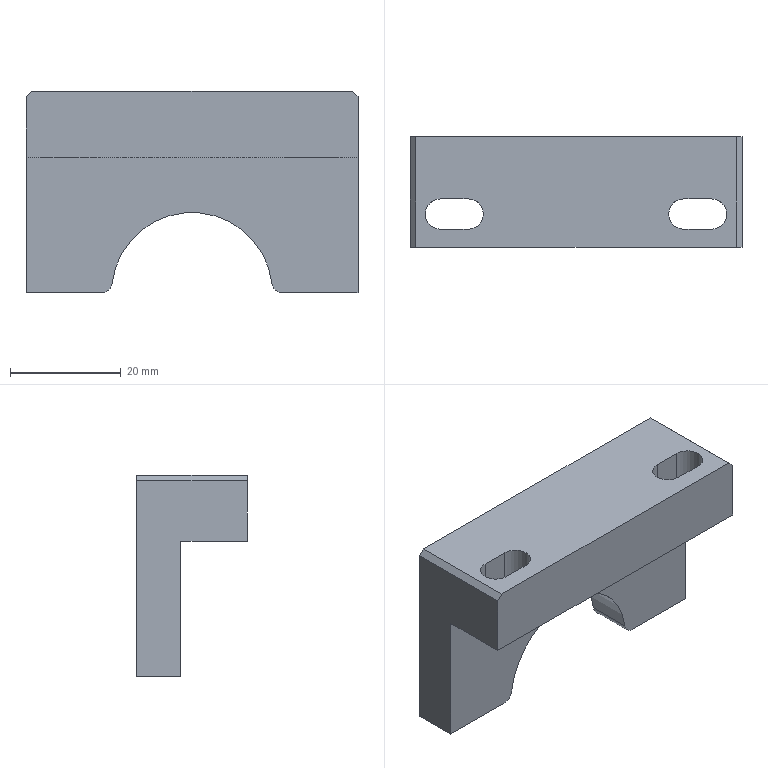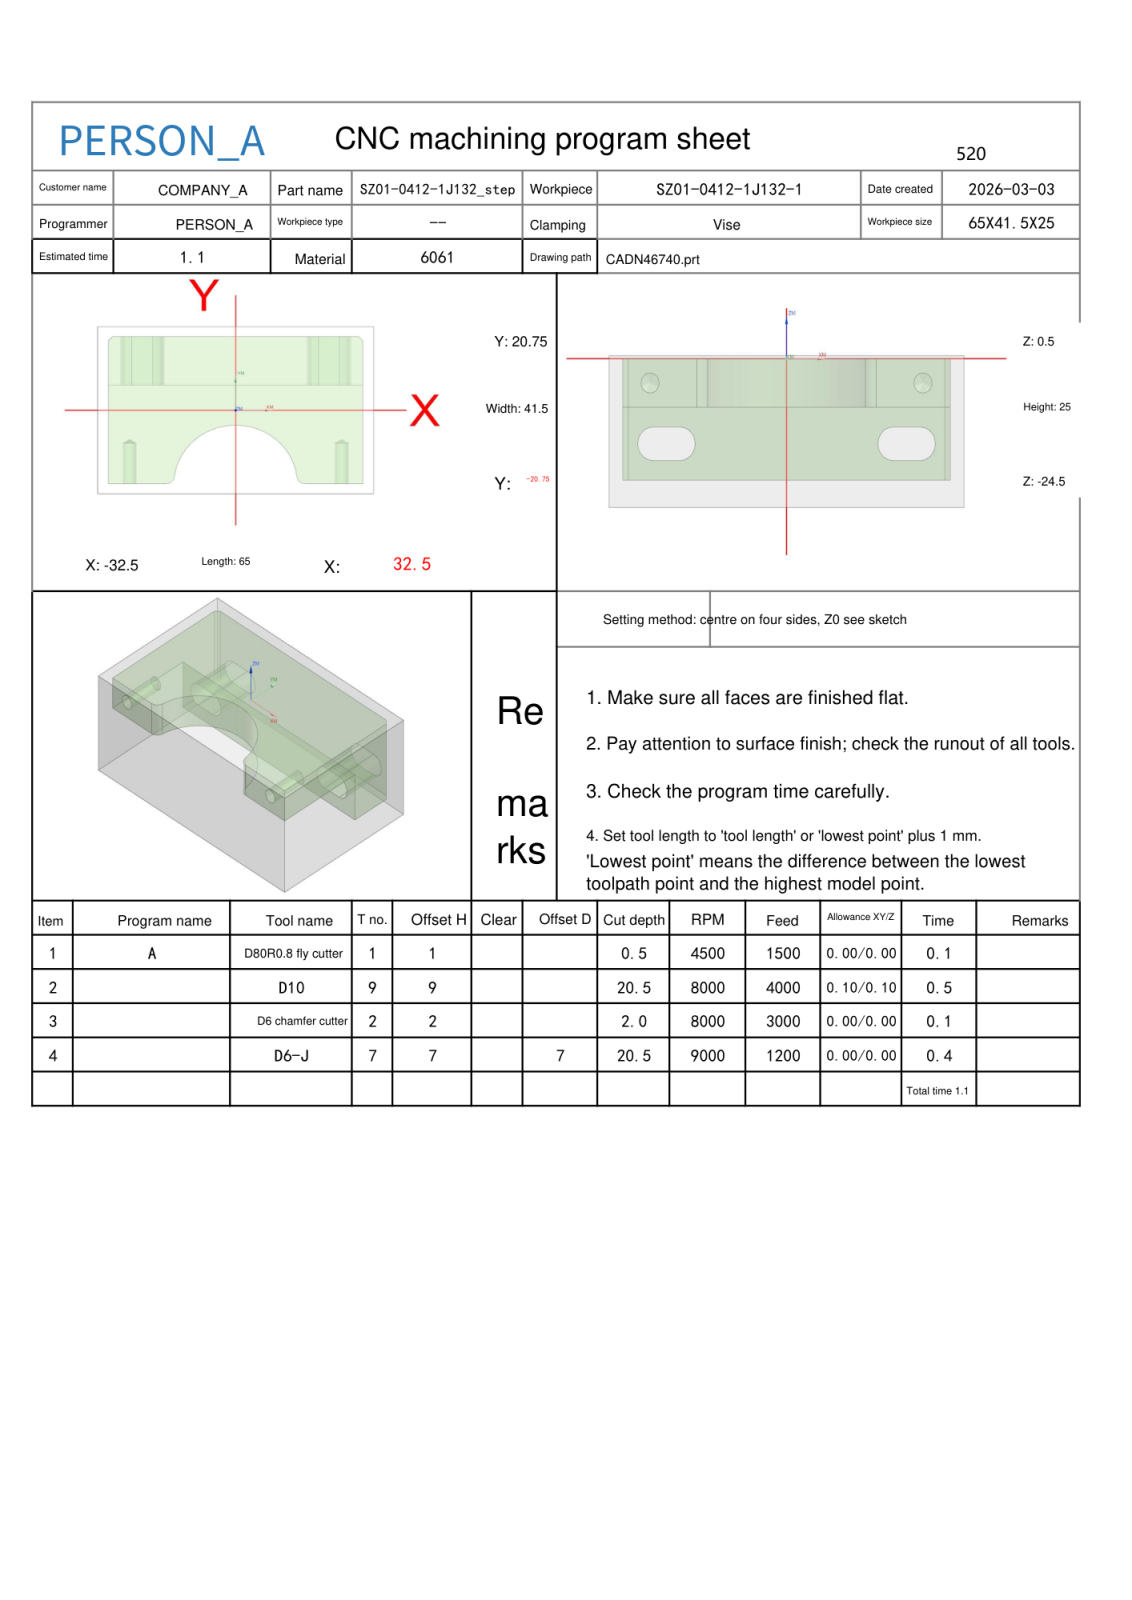NC program | NX | posted by the shop | part box 60 x 20 x 36.5 mm
Whole program:
%
O0001
(Machine time: 1.86 MIN)
(===Total Tool:4===)
(T1=D80R0.8 fly cutter D=80.  R=0.8  D-  H01 Z=0.    )
(T9=D10     D=10.  R=0.   D-  H09 Z=-20.  )
(T2=D6 chamfer cutter   D=6.   R=0.   D-  H02 Z=-1.5  )
(T7=D6-J    D=6.   R=0.   D7  H07 Z=-20.  )
G80 G90 G17 G49 G40
G91 G28 Z0
M01
N1 T01 M06
(D80R0.8 fly cutter  D=80. R=0.8 H=01 ce=0.00 di=0.00)
G00 G90 G54 X-75. Y0.0 M03 S4500
G43 H01 Z50.
M08
Z2.
G01 Z0.0 F1500.
X-70.
X70.
X75.
Z2.
G00 Z50.
G91 G28 Z0.0
M05
M09
G91 G28 Z0.0
M01
N2 T09 M06
(D10  D=10. R=0. H=09 ce=0.10 di=0.10)
G00 G90 G54 X-1.014 Y31.181 M03 S8000
G43 H09 Z50.
M08
Z-18.
G01 X-.995 Y31.082 Z-18.625 F4000.
X-.977 Y30.984 Z-18.872
X-.958 Y30.886 Z-19.054
X-.939 Y30.788 Z-19.2
X-.921 Y30.689 Z-19.323
X-.902 Y30.591 Z-19.428
X-.883 Y30.493 Z-19.52
X-.865 Y30.395 Z-19.6
X-.846 Y30.296 Z-19.67
X-.827 Y30.198 Z-19.732
X-.809 Y30.1 Z-19.786
X-.79 Y30.002 Z-19.833
X-.771 Y29.903 Z-19.874
X-.753 Y29.805 Z-19.908
X-.734 Y29.707 Z-19.936
X-.715 Y29.609 Z-19.96
X-.697 Y29.511 Z-19.977
X-.678 Y29.412 Z-19.99
X-.659 Y29.314 Z-19.997
X-.641 Y29.216 Z-20.
X-.239 Y27.102
G03 X.02 Y26.75 I.505 J.101
X3.834 Y26.112 I4.014 J12.271
X14.004 Y25.931 I10.17 J285.72
X17.328 Y25.95 I0.0 J285.901
G02 X22.505 Y25.974 I5.176 J-566.013
X30.847 Y25.912 I0.0 J-566.037
X35.808 Y22.571 I-.576 J-6.208
X37.387 Y16.992 I-12.592 J-6.578
X37.711 Y8.503 I-111.018 J-8.489
X37.695 Y6.6 I-111.342 J0.0
G01 X37.676 Y-18.9
G02 X34.409 Y-23.999 I-6.192 J.371
X28.685 Y-25.642 I-6.663 J12.425
X20.198 Y-25.962 I-8.487 J112.43
X18.294 Y-25.945 I0.0 J112.75
G01 X-30.63 Y-25.928
G02 X-35.719 Y-22.702 I.352 J6.181
X-37.387 Y-16.973 I12.246 J6.672
X-37.7 Y-9.187 I96.703 J7.786
X-37.692 Y-7.942 I97.015 J0.0
G01 X-37.676 Y18.9
G02 X-34.447 Y23.972 I6.185 J-.374
X-28.889 Y25.618 I6.599 J-12.074
X-20.788 Y25.956 I8.1 J-97.034
X-19.218 Y25.943 I0.0 J-97.371
X-12.284 Y25.971 I6.934 J-881.187
X-2.439 Y25.916 I0.0 J-881.214
G03 X6.567 Y25.245 I14.435 J133.079
X21.95 Y25.126 I15.383 J989.867
X28.108 Y25.145 I0.0 J989.986
G02 X34.603 Y21.21 I-.184 J-7.63
X36.473 Y15.222 I-13.036 J-7.357
X36.899 Y6.533 I-88.401 J-8.69
X36.888 Y5.156 I-88.827 J0.0
G01 X36.878 Y-16.757
G02 X32.777 Y-22.959 I-7.676 J.618
X26.519 Y-24.774 I-7.551 J14.34
X17.602 Y-25.155 I-8.918 J104.227
X15.971 Y-25.142 I0.0 J104.608
G01 X-28.487 Y-25.129
G02 X-34.704 Y-21.033 I.6 J7.678
X-36.532 Y-14.698 I14.384 J7.582
X-36.904 Y-5.801 I106.207 J8.896
X-36.893 Y-4.229 I106.579 J0.0
G01 X-36.879 Y16.737
G02 X-33.057 Y22.788 I7.611 J-.575
X-27.079 Y24.708 I7.365 J-12.666
X-19.035 Y25.132 I8.044 J-75.929
X-18.294 Y25.129 I0.0 J-76.354
X-11.995 Y25.164 I6.3 J-560.555
X-3.675 Y25.103 I0.0 J-560.59
G03 X6.265 Y24.482 I27.961 J367.714
X22.104 Y24.326 I15.839 J805.883
X26.268 Y24.337 I0.0 J806.039
G02 X30.598 Y23.063 I-.108 J-8.365
X32.829 Y21.648 I-1.556 J-4.922
X34.641 Y19.364 I-5.043 J-5.86
X35.582 Y14.955 I-17.95 J-6.134
X36.112 Y4.461 I-103.61 J-10.494
X36.093 Y2.493 I-104.14 J0.0
X36.121 Y-4.832 I-944.209 J-7.326
X36.068 Y-14.846 I-944.237 J0.0
X35.073 Y-18.453 I-8.82 J.492
G01 X34.926 Y-19.57
X34.417 Y-20.8
X33.606 Y-21.856
X32.55 Y-22.667
X31.32 Y-23.176
G02 X19.21 Y-24.313 I-12.83 J71.616
G01 X8.331 Y-24.349
X-26.289 Y-24.333
G02 X-30.191 Y-23.325 I.171 J8.716
G01 X-31.32 Y-23.176
X-32.55 Y-22.667
X-33.606 Y-21.856
X-34.417 Y-20.8
G02 X-35.145 Y-18.268 I6.23 J3.162
X-36.057 Y-7.678 I70.414 J11.403
G01 X-36.099 Y4.241
G02 X-36.123 Y8.231 I332.132 J3.99
X-36.052 Y15.1 I332.156 J0.0
X-34.818 Y18.836 I8.257 J-.655
X-33.606 Y20.857 I4.477 J-1.312
X-31.486 Y22.703 I7.177 J-6.102
X-28.417 Y23.572 I4.288 J-9.287
X-19.095 Y24.312 I9.951 J-66.268
X-12.541 Y24.363 I6.554 J-421.66
X-3.416 Y24.264 I0.0 J-421.711
G03 X15.543 Y23.546 I18.959 J249.717
X17.735 Y23.555 I0.0 J250.435
G02 X20.074 Y23.572 I2.339 J-160.329
X25.168 Y23.491 I0.0 J-160.346
G01 X26.223 Y23.35
X29.025
X30.297 Y23.185
X30.668 Y23.035
X30.297 Y23.185
X29.025 Y23.35
X1.555 Y23.373
G03 X-11.967 Y23.724 I-13.522 J-260.677
X-22.674 Y23.504 I0.0 J-261.028
G01 X-24.721 Y23.35
X-29.023
X-30.297 Y23.185
X-29.023 Y23.35
X2.399
G03 X2.779 Y23.525 I-.006 J.513
G01 X3.45 Y24.312
X4.729 Y25.812 Z-19.9
X5.155 Y26.311
X5.217 Y26.372
X5.288 Y26.421
X5.366 Y26.457
X5.45 Y26.479
X5.536 Y26.487
X31.253
X31.455 Y26.48
X31.656 Y26.461
X31.855 Y26.429
X32.051 Y26.384
X32.245 Y26.326
X32.434 Y26.256
X32.618 Y26.174
X32.797 Y26.081
X32.969 Y25.976
X33.134 Y25.86
X33.292 Y25.734
X33.441 Y25.598
X33.581 Y25.452
X36.132 Y22.626
X36.178 Y22.566
X36.215 Y22.5
X36.242 Y22.428
X36.257 Y22.354
X36.261 Y22.278
X36.253 Y22.202
X36.234 Y22.129
X36.099 Y21.736
X35.459 Y19.871 Z-20.
X34.989 Y18.486
X35.1 Y17.264
G03 X35.096 Y15.815 I269.611 J-1.449
X35.251 Y6.666 I269.615 J0.0
G02 X35.314 Y-3.77 I-871.941 J-10.435
X35.264 Y-13.074 I-872.004 J0.0
G01 X35.1 Y-14.475
G02 X35.123 Y-16.057 I-54.463 J-1.582
X35.068 Y-18.49 I-54.486 J0.0
G01 X35.1 Y-18.252
Y12.165
G02 X35.6 Y12.665 I.5 J0.0
X36.013 Y12.446 I0.0 J-.5
G01 X36.447 Y11.81
X37.557 Y10.18 Z-19.9
X38.15 Y9.309
X38.187 Y9.244
X38.215 Y9.175
X38.231 Y9.102
X38.237 Y9.028
Y-21.997
X38.23 Y-22.147
X38.209 Y-22.297
X38.173 Y-22.443
X38.124 Y-22.586
X38.062 Y-22.723
X37.987 Y-22.854
X37.901 Y-22.977
X37.803 Y-23.092
X37.694 Y-23.196
X37.576 Y-23.291
X37.45 Y-23.373
X37.317 Y-23.443
X35.367 Y-24.356
X35.298 Y-24.382
X35.226 Y-24.398
X35.152 Y-24.403
X35.079 Y-24.397
X35.007 Y-24.38
X34.576 Y-24.246
X32.693 Y-23.66 Z-20.
X31.226 Y-23.209
X29.998 Y-23.35
G03 X27.976 Y-23.343 I-2.023 J-280.372
X18.537 Y-23.502 I0.0 J-280.38
G01 X7.418 Y-23.548
X-24.567 Y-23.528
G02 X-26.225 Y-23.35 I4.859 J53.157
X-27.806 Y-23.373 I-1.582 J54.493
X-30.24 Y-23.318 I0.0 J54.516
G03 X-27.806 Y-23.373 I2.433 J54.462
X-26.225 Y-23.35 I0.0 J54.516
G01 X-16.43
G02 X-8.791 Y-22.914 I7.639 J-66.762
X-7.826 Y-22.921 I0.0 J-67.198
G01 X13.95 Y-22.909
G03 X16.378 Y-23.35 I2.544 J7.11
G01 X24.058
X16.378
G02 X13.378 Y-22.689 I.38 J8.862
G03 X8.341 Y-22.183 I-5.036 J-24.806
G01 X8.194
G03 X-1.001 Y-22.09 I-9.194 J-455.079
X-11.902 Y-22.221 I0.0 J-455.172
X-12.81 Y-22.316 I.059 J-4.951
G01 X-13.571 Y-22.75
X-14.969 Y-23.198
G03 X-12.669 Y-22.239 I-1.724 J7.368
G02 X-8.86 Y-21.62 I3.959 J-12.333
X.133 Y-21.452 I8.993 J-240.391
X9.795 Y-21.646 I0.0 J-240.559
X12.26 Y-21.966 I-.73 J-15.266
G03 X13.948 Y-22.888 I4.326 J5.915
G02 X12.031 Y-21.806 I2.886 J7.348
G03 X8.287 Y-20.956 I-4.278 J-10.178
X-.545 Y-20.662 I-8.832 J-132.62
X-3.41 Y-20.693 I0.0 J-132.914
X-4.321 Y-20.685 I-.912 J-48.82
X-10.702 Y-21.103 I0.0 J-48.829
X-11.508 Y-21.326 I.449 J-3.2
G02 X-12.783 Y-22.3 I-3.746 J3.578
G03 X-11.385 Y-21.224 I-3.037 J5.389
G02 X-8.045 Y-20.354 I3.85 J-7.936
X-.059 Y-20.038 I7.986 J-100.6
X3.415 Y-20.098 I0.0 J-100.916
G01 X3.664 Y-20.097
G02 X10.153 Y-20.696 I0.0 J-35.459
X11.273 Y-21.099 I-.371 J-2.784
G03 X12.296 Y-21.979 I4.434 J4.121
G02 X11.028 Y-20.863 I5.352 J7.361
G03 X7.741 Y-19.767 I-4.184 J-7.076
X.032 Y-19.277 I-7.708 J-60.321
X-1.503 Y-19.296 I0.0 J-60.811
X-2.306 Y-19.289 I-.804 J-43.621
X-8.815 Y-19.777 I0.0 J-43.629
X-10.676 Y-20.367 I.73 J-5.531
G02 X-11.497 Y-21.315 I-3.521 J2.218
G03 X-10.664 Y-20.332 I-2.483 J2.948
G02 X-7.94 Y-19.232 I3.56 J-4.89
X-1.171 Y-18.681 I6.769 J-41.337
X-.17 Y-18.693 I0.0 J-41.888
X.837 Y-18.682 I1.007 J-43.524
X8.068 Y-19.286 I0.0 J-43.535
X10.518 Y-20.159 I-1.033 J-6.775
G01 X11.27 Y-21.095
G03 X10.016 Y-19.691 I-5.989 J-4.087
X6.215 Y-18.406 I-4.918 J-8.281
X-.505 Y-17.931 I-6.72 J-47.364
X-6.959 Y-18.369 I0.0 J-47.838
X-10.034 Y-19.377 I1.179 J-8.793
X-10.322 Y-19.872 I1.707 J-1.323
G01 X-10.704 Y-20.386
G03 X-10.09 Y-19.393 I-3.127 J2.62
G02 X-7.442 Y-18.07 I3.713 J-4.116
X-.903 Y-17.361 I6.539 J-29.8
X.055 Y-17.376 I0.0 J-30.509
X.639 Y-17.37 I.584 J-30.655
X7.531 Y-18.155 I0.0 J-30.66
X10.071 Y-19.341 I-1.413 J-6.339
G01 X10.434 Y-20.054
G03 X8.446 Y-18.056 I-3.15 J-1.145
X2.894 Y-16.804 I-6.406 J-15.464
X-.435 Y-16.641 I-3.329 J-33.914
X-6.49 Y-17.183 I0.0 J-34.077
X-9.641 Y-18.471 I1.328 J-7.748
X-10.165 Y-19.532 I9.988 J-5.598
G02 X-9.548 Y-18.314 I5.132 J-1.837
X-6.593 Y-16.797 I4.26 J-4.661
X-.298 Y-16.081 I6.295 J-27.319
X1.982 Y-16.174 I0.0 J-28.035
X8.153 Y-17.436 I-.519 J-18.246
X9.657 Y-18.423 I-1.893 J-4.526
G01 X10.059 Y-19.287
X9.578 Y-18.229
G03 X6.972 Y-16.501 I-4.214 J-3.525
X.122 Y-15.411 I-6.851 J-20.979
X-.354 Y-15.416 I0.0 J-22.069
X-1.016 Y-15.405 I-.663 J-20.604
X-7.259 Y-16.373 I0.0 J-20.615
X-9.509 Y-17.767 I1.437 J-4.834
G01 X-9.709 Y-18.541
G02 X-8.531 Y-16.696 I2.33 J-.188
X-3.899 Y-15.129 I5.79 J-9.49
X-.267 Y-14.857 I3.632 J-24.065
X6.266 Y-15.75 I0.0 J-24.338
X9.42 Y-17.571 I-1.791 J-6.746
X9.721 Y-18.549 I-2.717 J-1.373
G03 X9.194 Y-17.107 I-3.311 J-.393
X5.948 Y-15.119 I-5.073 J-4.64
X-.341 Y-14.19 I-6.288 J-20.8
X-6.25 Y-15.009 I0.0 J-21.729
X-9.25 Y-16.753 I1.785 J-6.52
X-9.544 Y-17.818 I3.828 J-1.632
G02 X-9.2 Y-16.592 I4.419 J-.58
X-6.587 Y-14.731 I4.359 J-3.353
X-.434 Y-13.672 I6.153 J-17.351
X.919 Y-13.722 I0.0 J-18.409
X7.372 Y-15.219 I-.316 J-16.017
X9.315 Y-16.821 I-1.962 J-4.36
G01 X9.516 Y-17.695
G03 X9.052 Y-16.226 I-4.044 J-.47
X5.969 Y-14.091 I-5.111 J-4.089
X-.317 Y-13.024 I-6.286 J-17.985
X-6.147 Y-13.939 I0.0 J-19.051
X-9.06 Y-15.787 I1.939 J-6.275
X-9.327 Y-16.855 I13.275 J-3.88
G02 X-8.98 Y-15.57 I4.852 J-.621
X-6.238 Y-13.569 I4.599 J-3.423
X-.235 Y-12.514 I6.003 J-16.536
X2.229 Y-12.687 I0.0 J-17.592
X7.904 Y-14.613 I-1.087 J-12.528
X9.123 Y-15.874 I-1.924 J-3.079
G01 X9.305 Y-16.749
G03 X8.854 Y-15.222 I-4.366 J-.459
X5.846 Y-13.014 I-5.188 J-3.914
X-.288 Y-11.885 I-6.134 J-16.1
X-6.128 Y-12.904 I0.0 J-17.229
X-8.64 Y-14.527 I2.117 J-6.034
X-9.118 Y-15.9 I4.608 J-2.37
G02 X-8.065 Y-13.747 I4.041 J-.642
X-3.718 Y-11.756 I5.807 J-6.938
X-.223 Y-11.385 I3.495 J-16.28
X6.267 Y-12.702 I0.0 J-16.651
X8.609 Y-14.409 I-2.476 J-5.859
X9.102 Y-15.768 I-18.427 J-7.445
G03 X8.231 Y-13.733 I-6.594 J-1.619
X4.733 Y-11.568 I-5.555 J-5.067
X-.247 Y-10.767 I-4.98 J-15.069
X-6.051 Y-11.866 I0.0 J-15.871
X-7.702 Y-12.842 I2.975 J-6.916
X-8.613 Y-14.463 I4.56 J-3.631
G02 X-6.835 Y-11.996 I5.094 J-1.798
X-1.671 Y-10.371 I5.743 J-9.233
X-.088 Y-10.286 I1.583 J-14.686
X6.3 Y-11.739 I0.0 J-14.771
X7.698 Y-12.776 I-1.459 J-3.428
G01 X8.531 Y-14.208
G03 X6.635 Y-11.627 I-7.515 J-3.534
X1.729 Y-9.833 I-5.847 J-8.379
X-.291 Y-9.688 I-2.02 J-14.051
X-5.719 Y-10.767 I0.0 J-14.196
X-7.622 Y-12.723 I4.998 J-6.764
G02 X-3.947 Y-9.822 I6.414 J-4.347
X-.011 Y-9.239 I3.935 J-12.981
X4.621 Y-10.055 I0.0 J-13.565
X7.043 Y-11.997 I-3.838 J-7.268
G03 X4.621 Y-10.055 I-6.327 J-5.409
G01 X3.854 Y-9.627
G03 X-.092 Y-8.823 I-3.946 J-9.278
X-1.34 Y-8.9 I0.0 J-10.083
X-4.673 Y-10.042 I1.783 J-10.643
G01 X-5.199 Y-10.406
G03 X-5.414 Y-10.82 I.291 J-.414
G01 X-5.413 Y-10.847
X-5.362 Y-11.708
X-5.244 Y-13.676 Z-19.9
X-5.183 Y-14.686
X-5.185 Y-14.765
X-5.199 Y-14.842
X-6.381 Y-19.367
X-6.471 Y-19.688
X-6.575 Y-20.005
X-6.692 Y-20.317
X-6.821 Y-20.624
X-6.963 Y-20.926
X-7.117 Y-21.222
X-7.282 Y-21.511
X-7.46 Y-21.794
X-7.649 Y-22.068
X-7.848 Y-22.335
X-8.059 Y-22.594
X-8.28 Y-22.843
X-8.511 Y-23.084
X-8.725 Y-23.298
X-8.987 Y-23.55
X-9.257 Y-23.792
X-9.537 Y-24.023
X-9.825 Y-24.244
X-10.121 Y-24.453
X-10.425 Y-24.652
X-10.736 Y-24.838
X-11.053 Y-25.013
X-11.378 Y-25.176
X-11.708 Y-25.327
X-12.043 Y-25.465
X-12.384 Y-25.59
X-12.729 Y-25.703
X-12.784 Y-25.72
X-13.255 Y-25.857
X-13.729 Y-25.981
X-14.206 Y-26.094
X-14.686 Y-26.194
X-15.168 Y-26.281
X-15.652 Y-26.356
X-16.139 Y-26.419
X-16.626 Y-26.469
X-17.115 Y-26.506
X-17.604 Y-26.53
X-33.859 Y-27.132
X-33.991 Y-27.13
X-34.122 Y-27.114
X-34.251 Y-27.085
X-34.377 Y-27.042
X-34.497 Y-26.987
X-34.61 Y-26.92
X-34.717 Y-26.841
X-34.814 Y-26.751
X-34.902 Y-26.652
X-34.978 Y-26.544
X-35.043 Y-26.429
X-35.096 Y-26.308
X-36.106 Y-23.617
X-36.128 Y-23.539
X-36.137 Y-23.458
X-36.133 Y-23.376
X-36.116 Y-23.296
X-35.978 Y-22.843
X-35.405 Y-20.956 Z-20.
X-34.959 Y-19.473
X-35.1 Y-18.248
G03 X-35.093 Y-16.258 I-279.481 J1.991
X-35.251 Y-6.845 I-279.488 J0.0
G02 X-35.316 Y3.496 I834.454 J10.341
X-35.26 Y13.136 I834.518 J0.0
G01 X-35.1 Y14.458
Y17.267
G02 X-34.811 Y18.858 I5.078 J-.1
G03 X-35.1 Y17.267 I4.79 J-1.691
G01 Y-12.342
G02 X-35.547 Y-12.843 I-.506 J.001
G01 X-37.565 Y-13.077
X-37.664 Y-13.089 Z-19.997
X-37.763 Y-13.1 Z-19.99
X-37.863 Y-13.112 Z-19.977
X-37.962 Y-13.123 Z-19.96
X-38.061 Y-13.135 Z-19.936
X-38.161 Y-13.146 Z-19.908
X-38.26 Y-13.158 Z-19.874
X-38.359 Y-13.169 Z-19.833
X-38.459 Y-13.181 Z-19.786
X-38.558 Y-13.192 Z-19.732
X-38.657 Y-13.204 Z-19.67
X-38.757 Y-13.215 Z-19.6
X-38.856 Y-13.227 Z-19.52
X-38.955 Y-13.238 Z-19.428
X-39.055 Y-13.25 Z-19.323
X-39.154 Y-13.261 Z-19.2
X-39.253 Y-13.273 Z-19.054
X-39.353 Y-13.284 Z-18.872
X-39.452 Y-13.296 Z-18.625
X-39.551 Y-13.307 Z-18.
G00 Z50.
G91 G28 Z0.0
M05
M09
G91 G28 Z0.0
M01
N3 T02 M06
(D6 chamfer cutter  D=6. R=0. H=02 ce=0.00 di=0.00)
G00 G90 G54 X-.25 Y20.378 M03 S8000
G43 H02 Z50.
M08
Z2.099
G01 Z-1.5 F3000.
G03 X-.33 Y20.078 I.52 J-.3
X-.03 Y19.558 I.6 J0.0
G01 X0.0 Y19.55
X29.
X29.254 Y19.525
X29.497 Y19.451
X29.722 Y19.331
X29.919 Y19.169
X30.919 Y18.169
X31.081 Y17.972
X31.201 Y17.747
X31.275 Y17.504
X31.3 Y17.25
Y-18.25
G02 X30. Y-19.55 I-1.3 J0.0
G01 X16.429
G02 X13.153 Y-16.649 I0.0 J3.3
G03 X0.0 Y-5. I-13.153 J-1.601
X-13.153 Y-16.649 I0.0 J-13.25
G02 X-16.429 Y-19.55 I-3.276 J.399
G01 X-30.
G02 X-31.3 Y-18.25 I0.0 J1.3
G01 Y17.25
X-31.275 Y17.504
X-31.201 Y17.747
X-31.081 Y17.972
X-30.919 Y18.169
X-29.919 Y19.169
X-29.722 Y19.331
X-29.497 Y19.451
X-29.254 Y19.525
X-29. Y19.55
X0.0
X.03 Y19.558
G03 X.33 Y20.078 I-.3 J.52
X.25 Y20.378 I-.6 J0.0
G01 Z2.099
G00 Z50.
G91 G28 Z0.0
M05
M09
G91 G28 Z0.0
M01
N4 T07 M06
(D6-J  D=6. R=0. H=07 ce=0.00 di=0.00)
G00 G90 G54 X-30.017 Y22.323 M03 S9000
G43 H07 Z50.
M08
Z-9.5
G01 Z-10. F1200.
G41 D07
X-29.992 Y22.125
G03 X-29. Y21.25 I.992 J.125
G01 X29.
G02 X31.121 Y20.371 I0.0 J-3.
G01 X32.121 Y19.371
G02 X33. Y17.25 I-2.121 J-2.121
G01 Y-18.25
G02 X30. Y-21.25 I-3. J0.0
G01 X16.429
G02 X11.465 Y-16.854 I0.0 J5.
G03 X0.0 Y-6.7 I-11.465 J-1.396
X-11.465 Y-16.854 I0.0 J-11.55
G02 X-16.429 Y-21.25 I-4.963 J.604
G01 X-30.
G02 X-33. Y-18.25 I0.0 J3.
G01 Y17.25
G02 X-32.121 Y19.371 I3. J0.0
G01 X-31.121 Y20.371
G02 X-29. Y21.25 I2.121 J-2.121
G01 X-28.5
G03 X-27.5 Y22.25 I0.0 J1.
G01 G40 Y22.45
Z-9.5
G00 Z50.
X-30.017 Y22.323
Z-19.5
G01 Z-20.
G41 D07
X-29.992 Y22.125
G03 X-29. Y21.25 I.992 J.125
G01 X29.
G02 X31.121 Y20.371 I0.0 J-3.
G01 X32.121 Y19.371
G02 X33. Y17.25 I-2.121 J-2.121
G01 Y-18.25
G02 X30. Y-21.25 I-3. J0.0
G01 X16.429
G02 X11.465 Y-16.854 I0.0 J5.
G03 X0.0 Y-6.7 I-11.465 J-1.396
X-11.465 Y-16.854 I0.0 J-11.55
G02 X-16.429 Y-21.25 I-4.963 J.604
G01 X-30.
G02 X-33. Y-18.25 I0.0 J3.
G01 Y17.25
G02 X-32.121 Y19.371 I3. J0.0
G01 X-31.121 Y20.371
G02 X-29. Y21.25 I2.121 J-2.121
G01 X-28.5
G03 X-27.5 Y22.25 I0.0 J1.
G01 G40 Y22.45
Z-19.5
G00 Z50.
M05
M09
G91 G28 Z0.0
G91 G28 Y0.0
M30
%